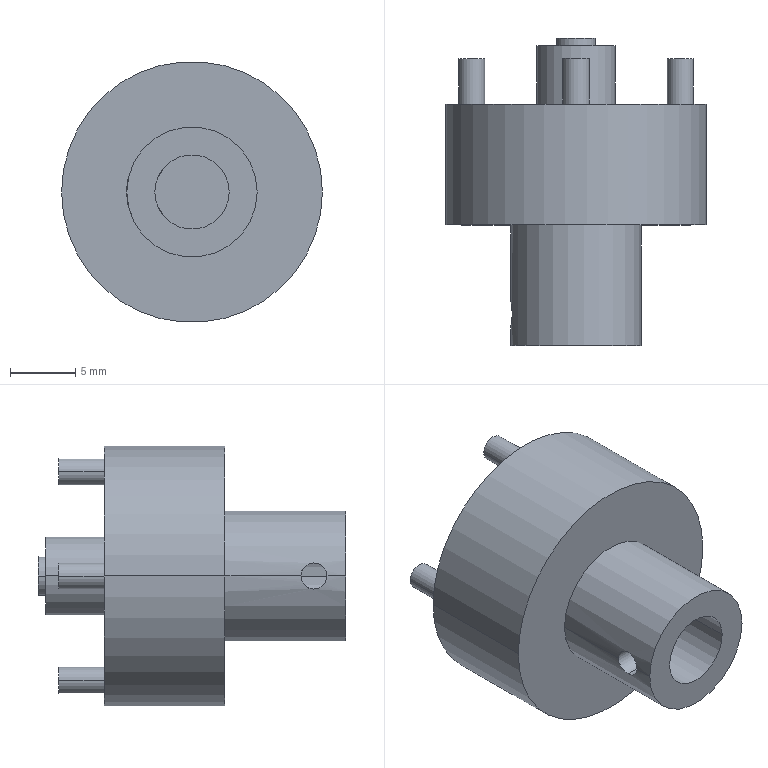Part | SolidWorks | features BaseBody 1 | 1 solid | 30 faces | box 20 x 23.55 x 20 mm | volume 3677 mm3 | cylinder 20 | plane 10 | commonest cylinder face diameters 2 x10 3 x2 5.7 x2 6 x2 10 x2 20 x2
STEP:
#1=CARTESIAN_POINT('',(7.,12.825,0.));
#2=VERTEX_POINT('',#1);
#3=CARTESIAN_POINT('',(9.,12.825,0.));
#4=VERTEX_POINT('',#3);
#5=CARTESIAN_POINT('',(8.,12.825,0.));
#6=DIRECTION('',(0.,1.,0.));
#7=DIRECTION('',(-1.,0.,0.));
#8=AXIS2_PLACEMENT_3D('',#5,#6,#7);
#9=CIRCLE('',#8,1.);
#10=EDGE_CURVE('',#2,#4,#9,.T.);
#11=ORIENTED_EDGE('',*,*,#10,.F.);
#12=CARTESIAN_POINT('',(7.,9.325,0.));
#13=VERTEX_POINT('',#12);
#14=CARTESIAN_POINT('',(7.,12.825,0.));
#15=DIRECTION('',(0.,-1.,0.));
#16=VECTOR('',#15,1000.);
#17=LINE('',#14,#16);
#18=EDGE_CURVE('',#2,#13,#17,.T.);
#19=ORIENTED_EDGE('',*,*,#18,.T.);
#20=CARTESIAN_POINT('',(9.,9.325,0.));
#21=VERTEX_POINT('',#20);
#22=CARTESIAN_POINT('',(8.,9.325,0.));
#23=DIRECTION('',(0.,1.,0.));
#24=DIRECTION('',(-1.,0.,0.));
#25=AXIS2_PLACEMENT_3D('',#22,#23,#24);
#26=CIRCLE('',#25,1.);
#27=EDGE_CURVE('',#13,#21,#26,.T.);
#28=ORIENTED_EDGE('',*,*,#27,.T.);
#29=CARTESIAN_POINT('',(9.,12.825,0.));
#30=DIRECTION('',(0.,-1.,0.));
#31=VECTOR('',#30,1000.);
#32=LINE('',#29,#31);
#33=EDGE_CURVE('',#4,#21,#32,.T.);
#34=ORIENTED_EDGE('',*,*,#33,.F.);
#35=EDGE_LOOP('',(#11,#19,#28,#34));
#36=FACE_OUTER_BOUND('',#35,.T.);
#37=CARTESIAN_POINT('',(8.,12.825,0.));
#38=DIRECTION('',(0.,-1.,0.));
#39=DIRECTION('',(1.,0.,0.));
#40=AXIS2_PLACEMENT_3D('',#37,#38,#39);
#41=CYLINDRICAL_SURFACE('',#40,1.);
#42=ADVANCED_FACE('',(#36),#41,.T.);
#43=CARTESIAN_POINT('',(-1.,12.825,-8.));
#44=VERTEX_POINT('',#43);
#45=CARTESIAN_POINT('',(1.,12.825,-8.));
#46=VERTEX_POINT('',#45);
#47=CARTESIAN_POINT('',(0.,12.825,-8.));
#48=DIRECTION('',(0.,1.,0.));
#49=DIRECTION('',(-1.,0.,0.));
#50=AXIS2_PLACEMENT_3D('',#47,#48,#49);
#51=CIRCLE('',#50,1.);
#52=EDGE_CURVE('',#44,#46,#51,.T.);
#53=ORIENTED_EDGE('',*,*,#52,.F.);
#54=CARTESIAN_POINT('',(-1.,9.325,-8.));
#55=VERTEX_POINT('',#54);
#56=CARTESIAN_POINT('',(-1.,12.825,-8.));
#57=DIRECTION('',(0.,-1.,0.));
#58=VECTOR('',#57,1000.);
#59=LINE('',#56,#58);
#60=EDGE_CURVE('',#44,#55,#59,.T.);
#61=ORIENTED_EDGE('',*,*,#60,.T.);
#62=CARTESIAN_POINT('',(1.,9.325,-8.));
#63=VERTEX_POINT('',#62);
#64=CARTESIAN_POINT('',(0.,9.325,-8.));
#65=DIRECTION('',(0.,1.,0.));
#66=DIRECTION('',(-1.,0.,0.));
#67=AXIS2_PLACEMENT_3D('',#64,#65,#66);
#68=CIRCLE('',#67,1.);
#69=EDGE_CURVE('',#55,#63,#68,.T.);
#70=ORIENTED_EDGE('',*,*,#69,.T.);
#71=CARTESIAN_POINT('',(1.,12.825,-8.));
#72=DIRECTION('',(0.,-1.,0.));
#73=VECTOR('',#72,1000.);
#74=LINE('',#71,#73);
#75=EDGE_CURVE('',#46,#63,#74,.T.);
#76=ORIENTED_EDGE('',*,*,#75,.F.);
#77=EDGE_LOOP('',(#53,#61,#70,#76));
#78=FACE_OUTER_BOUND('',#77,.T.);
#79=CARTESIAN_POINT('',(0.,12.825,-8.));
#80=DIRECTION('',(0.,-1.,0.));
#81=DIRECTION('',(1.,0.,0.));
#82=AXIS2_PLACEMENT_3D('',#79,#80,#81);
#83=CYLINDRICAL_SURFACE('',#82,1.);
#84=ADVANCED_FACE('',(#78),#83,.T.);
#85=CARTESIAN_POINT('',(-9.,12.825,0.));
#86=VERTEX_POINT('',#85);
#87=CARTESIAN_POINT('',(-7.,12.825,0.));
#88=VERTEX_POINT('',#87);
#89=CARTESIAN_POINT('',(-8.,12.825,0.));
#90=DIRECTION('',(0.,1.,0.));
#91=DIRECTION('',(-1.,0.,0.));
#92=AXIS2_PLACEMENT_3D('',#89,#90,#91);
#93=CIRCLE('',#92,1.);
#94=EDGE_CURVE('',#86,#88,#93,.T.);
#95=ORIENTED_EDGE('',*,*,#94,.F.);
#96=CARTESIAN_POINT('',(-9.,9.325,0.));
#97=VERTEX_POINT('',#96);
#98=CARTESIAN_POINT('',(-9.,12.825,0.));
#99=DIRECTION('',(0.,-1.,0.));
#100=VECTOR('',#99,1000.);
#101=LINE('',#98,#100);
#102=EDGE_CURVE('',#86,#97,#101,.T.);
#103=ORIENTED_EDGE('',*,*,#102,.T.);
#104=CARTESIAN_POINT('',(-7.,9.325,0.));
#105=VERTEX_POINT('',#104);
#106=CARTESIAN_POINT('',(-8.,9.325,0.));
#107=DIRECTION('',(0.,1.,0.));
#108=DIRECTION('',(-1.,0.,0.));
#109=AXIS2_PLACEMENT_3D('',#106,#107,#108);
#110=CIRCLE('',#109,1.);
#111=EDGE_CURVE('',#97,#105,#110,.T.);
#112=ORIENTED_EDGE('',*,*,#111,.T.);
#113=CARTESIAN_POINT('',(-7.,12.825,0.));
#114=DIRECTION('',(0.,-1.,0.));
#115=VECTOR('',#114,1000.);
#116=LINE('',#113,#115);
#117=EDGE_CURVE('',#88,#105,#116,.T.);
#118=ORIENTED_EDGE('',*,*,#117,.F.);
#119=EDGE_LOOP('',(#95,#103,#112,#118));
#120=FACE_OUTER_BOUND('',#119,.T.);
#121=CARTESIAN_POINT('',(-8.,12.825,0.));
#122=DIRECTION('',(0.,-1.,0.));
#123=DIRECTION('',(1.,0.,0.));
#124=AXIS2_PLACEMENT_3D('',#121,#122,#123);
#125=CYLINDRICAL_SURFACE('',#124,1.);
#126=ADVANCED_FACE('',(#120),#125,.T.);
#127=CARTESIAN_POINT('',(-1.,12.825,8.));
#128=VERTEX_POINT('',#127);
#129=CARTESIAN_POINT('',(1.,12.825,8.));
#130=VERTEX_POINT('',#129);
#131=CARTESIAN_POINT('',(0.,12.825,8.));
#132=DIRECTION('',(0.,1.,0.));
#133=DIRECTION('',(-1.,0.,0.));
#134=AXIS2_PLACEMENT_3D('',#131,#132,#133);
#135=CIRCLE('',#134,1.);
#136=EDGE_CURVE('',#128,#130,#135,.T.);
#137=ORIENTED_EDGE('',*,*,#136,.F.);
#138=CARTESIAN_POINT('',(-1.,9.325,8.));
#139=VERTEX_POINT('',#138);
#140=CARTESIAN_POINT('',(-1.,12.825,8.));
#141=DIRECTION('',(0.,-1.,0.));
#142=VECTOR('',#141,1000.);
#143=LINE('',#140,#142);
#144=EDGE_CURVE('',#128,#139,#143,.T.);
#145=ORIENTED_EDGE('',*,*,#144,.T.);
#146=CARTESIAN_POINT('',(1.,9.325,8.));
#147=VERTEX_POINT('',#146);
#148=CARTESIAN_POINT('',(0.,9.325,8.));
#149=DIRECTION('',(0.,1.,0.));
#150=DIRECTION('',(-1.,0.,0.));
#151=AXIS2_PLACEMENT_3D('',#148,#149,#150);
#152=CIRCLE('',#151,1.);
#153=EDGE_CURVE('',#139,#147,#152,.T.);
#154=ORIENTED_EDGE('',*,*,#153,.T.);
#155=CARTESIAN_POINT('',(1.,12.825,8.));
#156=DIRECTION('',(0.,-1.,0.));
#157=VECTOR('',#156,1000.);
#158=LINE('',#155,#157);
#159=EDGE_CURVE('',#130,#147,#158,.T.);
#160=ORIENTED_EDGE('',*,*,#159,.F.);
#161=EDGE_LOOP('',(#137,#145,#154,#160));
#162=FACE_OUTER_BOUND('',#161,.T.);
#163=CARTESIAN_POINT('',(0.,12.825,8.));
#164=DIRECTION('',(0.,-1.,0.));
#165=DIRECTION('',(1.,0.,0.));
#166=AXIS2_PLACEMENT_3D('',#163,#164,#165);
#167=CYLINDRICAL_SURFACE('',#166,1.);
#168=ADVANCED_FACE('',(#162),#167,.T.);
#169=CARTESIAN_POINT('',(-5.,-7.75,0.));
#170=VERTEX_POINT('',#169);
#171=CARTESIAN_POINT('',(-4.899,-6.75,1.));
#172=VERTEX_POINT('',#171);
#173=CARTESIAN_POINT('',(-5.,-7.75,0.));
#174=CARTESIAN_POINT('',(-5.,-7.75,0.1308));
#175=CARTESIAN_POINT('',(-4.995,-7.724,0.262));
#176=CARTESIAN_POINT('',(-4.976,-7.623,0.5045));
#177=CARTESIAN_POINT('',(-4.963,-7.55,0.6144));
#178=CARTESIAN_POINT('',(-4.936,-7.364,0.8002));
#179=CARTESIAN_POINT('',(-4.923,-7.254,0.8737));
#180=CARTESIAN_POINT('',(-4.905,-7.012,0.9739));
#181=CARTESIAN_POINT('',(-4.899,-6.881,1.));
#182=CARTESIAN_POINT('',(-4.899,-6.75,1.));
#183=B_SPLINE_CURVE_WITH_KNOTS('',3,(#173,#174,#175,#176,#177,#178,#179,#180,#181,#182),.UNSPECIFIED.,.F.,.F.,(4,2,2,2,4),(0.001568,0.001959,0.002351,0.002743,0.003134),.UNSPECIFIED.);
#184=EDGE_CURVE('',#170,#172,#183,.T.);
#185=ORIENTED_EDGE('',*,*,#184,.T.);
#186=CARTESIAN_POINT('',(-2.669,-6.75,1.));
#187=VERTEX_POINT('',#186);
#188=CARTESIAN_POINT('',(-11.,-6.75,1.));
#189=DIRECTION('',(1.,0.,0.));
#190=VECTOR('',#189,1000.);
#191=LINE('',#188,#190);
#192=EDGE_CURVE('',#172,#187,#191,.T.);
#193=ORIENTED_EDGE('',*,*,#192,.T.);
#194=CARTESIAN_POINT('',(-2.85,-7.75,0.));
#195=VERTEX_POINT('',#194);
#196=CARTESIAN_POINT('',(-2.669,-6.75,1.));
#197=CARTESIAN_POINT('',(-2.669,-6.881,1.));
#198=CARTESIAN_POINT('',(-2.679,-7.014,0.9734));
#199=CARTESIAN_POINT('',(-2.714,-7.255,0.873));
#200=CARTESIAN_POINT('',(-2.737,-7.365,0.7995));
#201=CARTESIAN_POINT('',(-2.785,-7.549,0.6148));
#202=CARTESIAN_POINT('',(-2.807,-7.623,0.5057));
#203=CARTESIAN_POINT('',(-2.84,-7.724,0.263));
#204=CARTESIAN_POINT('',(-2.85,-7.75,0.1318));
#205=CARTESIAN_POINT('',(-2.85,-7.75,0.));
#206=B_SPLINE_CURVE_WITH_KNOTS('',3,(#196,#197,#198,#199,#200,#201,#202,#203,#204,#205),.UNSPECIFIED.,.F.,.F.,(4,2,2,2,4),(0.003152,0.003545,0.003939,0.004333,0.004727),.UNSPECIFIED.);
#207=EDGE_CURVE('',#187,#195,#206,.T.);
#208=ORIENTED_EDGE('',*,*,#207,.T.);
#209=CARTESIAN_POINT('',(-2.669,-6.75,-1.));
#210=VERTEX_POINT('',#209);
#211=CARTESIAN_POINT('',(-2.85,-7.75,0.));
#212=CARTESIAN_POINT('',(-2.85,-7.75,-0.1318));
#213=CARTESIAN_POINT('',(-2.84,-7.723,-0.2641));
#214=CARTESIAN_POINT('',(-2.808,-7.623,-0.505));
#215=CARTESIAN_POINT('',(-2.784,-7.549,-0.6156));
#216=CARTESIAN_POINT('',(-2.737,-7.365,-0.7989));
#217=CARTESIAN_POINT('',(-2.714,-7.256,-0.8727));
#218=CARTESIAN_POINT('',(-2.679,-7.013,-0.9735));
#219=CARTESIAN_POINT('',(-2.669,-6.883,-1.));
#220=CARTESIAN_POINT('',(-2.669,-6.75,-1.));
#221=B_SPLINE_CURVE_WITH_KNOTS('',3,(#211,#212,#213,#214,#215,#216,#217,#218,#219,#220),.UNSPECIFIED.,.F.,.F.,(4,2,2,2,4),(0.004727,0.005121,0.005515,0.005909,0.006303),.UNSPECIFIED.);
#222=EDGE_CURVE('',#195,#210,#221,.T.);
#223=ORIENTED_EDGE('',*,*,#222,.T.);
#224=CARTESIAN_POINT('',(-4.899,-6.75,-1.));
#225=VERTEX_POINT('',#224);
#226=CARTESIAN_POINT('',(-11.,-6.75,-1.));
#227=DIRECTION('',(1.,0.,0.));
#228=VECTOR('',#227,1000.);
#229=LINE('',#226,#228);
#230=EDGE_CURVE('',#225,#210,#229,.T.);
#231=ORIENTED_EDGE('',*,*,#230,.F.);
#232=CARTESIAN_POINT('',(-4.899,-6.75,-1.));
#233=CARTESIAN_POINT('',(-4.899,-6.883,-1.));
#234=CARTESIAN_POINT('',(-4.905,-7.013,-0.9738));
#235=CARTESIAN_POINT('',(-4.923,-7.255,-0.8732));
#236=CARTESIAN_POINT('',(-4.937,-7.365,-0.7989));
#237=CARTESIAN_POINT('',(-4.963,-7.549,-0.6148));
#238=CARTESIAN_POINT('',(-4.976,-7.624,-0.5034));
#239=CARTESIAN_POINT('',(-4.995,-7.724,-0.2627));
#240=CARTESIAN_POINT('',(-5.,-7.75,-0.1309));
#241=CARTESIAN_POINT('',(-5.,-7.75,0.));
#242=B_SPLINE_CURVE_WITH_KNOTS('',3,(#232,#233,#234,#235,#236,#237,#238,#239,#240,#241),.UNSPECIFIED.,.F.,.F.,(4,2,2,2,4),(0.,0.0003919,0.0007838,0.001176,0.001568),.UNSPECIFIED.);
#243=EDGE_CURVE('',#225,#170,#242,.T.);
#244=ORIENTED_EDGE('',*,*,#243,.T.);
#245=EDGE_LOOP('',(#185,#193,#208,#223,#231,#244));
#246=FACE_OUTER_BOUND('',#245,.T.);
#247=CARTESIAN_POINT('',(-11.,-6.75,0.));
#248=DIRECTION('',(1.,0.,0.));
#249=DIRECTION('',(0.,0.,-1.));
#250=AXIS2_PLACEMENT_3D('',#247,#248,#249);
#251=CYLINDRICAL_SURFACE('',#250,1.);
#252=ADVANCED_FACE('',(#246),#251,.F.);
#253=CARTESIAN_POINT('',(-2.85,-4.325,0.));
#254=VERTEX_POINT('',#253);
#255=CARTESIAN_POINT('',(2.85,-4.325,0.));
#256=VERTEX_POINT('',#255);
#257=CARTESIAN_POINT('',(0.,-4.325,0.));
#258=DIRECTION('',(0.,-1.,0.));
#259=DIRECTION('',(1.,0.,0.));
#260=AXIS2_PLACEMENT_3D('',#257,#258,#259);
#261=CIRCLE('',#260,2.85);
#262=EDGE_CURVE('',#254,#256,#261,.T.);
#263=ORIENTED_EDGE('',*,*,#262,.F.);
#264=CARTESIAN_POINT('',(-2.85,-5.75,0.));
#265=VERTEX_POINT('',#264);
#266=CARTESIAN_POINT('',(-2.85,-4.325,0.));
#267=DIRECTION('',(0.,-1.,0.));
#268=VECTOR('',#267,1000.);
#269=LINE('',#266,#268);
#270=EDGE_CURVE('',#254,#265,#269,.T.);
#271=ORIENTED_EDGE('',*,*,#270,.T.);
#272=CARTESIAN_POINT('',(-2.669,-6.75,-1.));
#273=CARTESIAN_POINT('',(-2.669,-6.617,-1.));
#274=CARTESIAN_POINT('',(-2.679,-6.486,-0.9734));
#275=CARTESIAN_POINT('',(-2.714,-6.244,-0.8726));
#276=CARTESIAN_POINT('',(-2.738,-6.134,-0.7984));
#277=CARTESIAN_POINT('',(-2.784,-5.951,-0.6153));
#278=CARTESIAN_POINT('',(-2.808,-5.877,-0.5046));
#279=CARTESIAN_POINT('',(-2.84,-5.777,-0.2641));
#280=CARTESIAN_POINT('',(-2.85,-5.75,-0.1317));
#281=CARTESIAN_POINT('',(-2.85,-5.75,0.));
#282=B_SPLINE_CURVE_WITH_KNOTS('',3,(#272,#273,#274,#275,#276,#277,#278,#279,#280,#281),.UNSPECIFIED.,.F.,.F.,(4,2,2,2,4),(0.,0.0003941,0.0007881,0.001182,0.001576),.UNSPECIFIED.);
#283=EDGE_CURVE('',#210,#265,#282,.T.);
#284=ORIENTED_EDGE('',*,*,#283,.F.);
#285=ORIENTED_EDGE('',*,*,#222,.F.);
#286=CARTESIAN_POINT('',(-2.85,-9.175,0.));
#287=VERTEX_POINT('',#286);
#288=CARTESIAN_POINT('',(-2.85,-4.325,0.));
#289=DIRECTION('',(0.,-1.,0.));
#290=VECTOR('',#289,1000.);
#291=LINE('',#288,#290);
#292=EDGE_CURVE('',#195,#287,#291,.T.);
#293=ORIENTED_EDGE('',*,*,#292,.T.);
#294=CARTESIAN_POINT('',(2.85,-9.175,0.));
#295=VERTEX_POINT('',#294);
#296=CARTESIAN_POINT('',(0.,-9.175,0.));
#297=DIRECTION('',(0.,-1.,0.));
#298=DIRECTION('',(1.,0.,0.));
#299=AXIS2_PLACEMENT_3D('',#296,#297,#298);
#300=CIRCLE('',#299,2.85);
#301=EDGE_CURVE('',#287,#295,#300,.T.);
#302=ORIENTED_EDGE('',*,*,#301,.T.);
#303=CARTESIAN_POINT('',(2.85,-4.325,0.));
#304=DIRECTION('',(0.,-1.,0.));
#305=VECTOR('',#304,1000.);
#306=LINE('',#303,#305);
#307=EDGE_CURVE('',#256,#295,#306,.T.);
#308=ORIENTED_EDGE('',*,*,#307,.F.);
#309=EDGE_LOOP('',(#263,#271,#284,#285,#293,#302,#308));
#310=FACE_OUTER_BOUND('',#309,.T.);
#311=CARTESIAN_POINT('',(0.,-4.325,0.));
#312=DIRECTION('',(0.,-1.,0.));
#313=DIRECTION('',(1.,0.,0.));
#314=AXIS2_PLACEMENT_3D('',#311,#312,#313);
#315=CYLINDRICAL_SURFACE('',#314,2.85);
#316=ADVANCED_FACE('',(#310),#315,.F.);
#317=CARTESIAN_POINT('',(5.,0.075,0.));
#318=VERTEX_POINT('',#317);
#319=CARTESIAN_POINT('',(-5.,0.075,0.));
#320=VERTEX_POINT('',#319);
#321=CARTESIAN_POINT('',(0.,0.075,0.));
#322=DIRECTION('',(0.,-1.,0.));
#323=DIRECTION('',(1.,0.,0.));
#324=AXIS2_PLACEMENT_3D('',#321,#322,#323);
#325=CIRCLE('',#324,5.);
#326=EDGE_CURVE('',#318,#320,#325,.T.);
#327=ORIENTED_EDGE('',*,*,#326,.T.);
#328=CARTESIAN_POINT('',(-5.,-5.75,0.));
#329=VERTEX_POINT('',#328);
#330=CARTESIAN_POINT('',(-5.,-4.325,0.));
#331=DIRECTION('',(0.,-1.,0.));
#332=VECTOR('',#331,1000.);
#333=LINE('',#330,#332);
#334=EDGE_CURVE('',#320,#329,#333,.T.);
#335=ORIENTED_EDGE('',*,*,#334,.T.);
#336=CARTESIAN_POINT('',(-4.899,-6.75,1.));
#337=CARTESIAN_POINT('',(-4.899,-6.619,1.));
#338=CARTESIAN_POINT('',(-4.905,-6.487,0.9737));
#339=CARTESIAN_POINT('',(-4.923,-6.247,0.8738));
#340=CARTESIAN_POINT('',(-4.937,-6.135,0.7995));
#341=CARTESIAN_POINT('',(-4.963,-5.951,0.6152));
#342=CARTESIAN_POINT('',(-4.976,-5.877,0.505));
#343=CARTESIAN_POINT('',(-4.995,-5.776,0.2622));
#344=CARTESIAN_POINT('',(-5.,-5.75,0.1321));
#345=CARTESIAN_POINT('',(-5.,-5.75,0.));
#346=B_SPLINE_CURVE_WITH_KNOTS('',3,(#336,#337,#338,#339,#340,#341,#342,#343,#344,#345),.UNSPECIFIED.,.F.,.F.,(4,2,2,2,4),(0.003134,0.003526,0.003918,0.00431,0.004702),.UNSPECIFIED.);
#347=EDGE_CURVE('',#172,#329,#346,.T.);
#348=ORIENTED_EDGE('',*,*,#347,.F.);
#349=ORIENTED_EDGE('',*,*,#184,.F.);
#350=CARTESIAN_POINT('',(-5.,-9.175,0.));
#351=VERTEX_POINT('',#350);
#352=CARTESIAN_POINT('',(-5.,-4.325,0.));
#353=DIRECTION('',(0.,-1.,0.));
#354=VECTOR('',#353,1000.);
#355=LINE('',#352,#354);
#356=EDGE_CURVE('',#170,#351,#355,.T.);
#357=ORIENTED_EDGE('',*,*,#356,.T.);
#358=CARTESIAN_POINT('',(5.,-9.175,0.));
#359=VERTEX_POINT('',#358);
#360=CARTESIAN_POINT('',(0.,-9.175,0.));
#361=DIRECTION('',(0.,-1.,0.));
#362=DIRECTION('',(1.,0.,0.));
#363=AXIS2_PLACEMENT_3D('',#360,#361,#362);
#364=CIRCLE('',#363,5.);
#365=EDGE_CURVE('',#359,#351,#364,.T.);
#366=ORIENTED_EDGE('',*,*,#365,.F.);
#367=CARTESIAN_POINT('',(5.,-4.325,0.));
#368=DIRECTION('',(0.,-1.,0.));
#369=VECTOR('',#368,1000.);
#370=LINE('',#367,#369);
#371=EDGE_CURVE('',#318,#359,#370,.T.);
#372=ORIENTED_EDGE('',*,*,#371,.F.);
#373=EDGE_LOOP('',(#327,#335,#348,#349,#357,#366,#372));
#374=FACE_OUTER_BOUND('',#373,.T.);
#375=CARTESIAN_POINT('',(0.,-4.325,0.));
#376=DIRECTION('',(0.,-1.,0.));
#377=DIRECTION('',(1.,0.,0.));
#378=AXIS2_PLACEMENT_3D('',#375,#376,#377);
#379=CYLINDRICAL_SURFACE('',#378,5.);
#380=ADVANCED_FACE('',(#374),#379,.T.);
#381=CARTESIAN_POINT('',(10.,9.325,0.));
#382=VERTEX_POINT('',#381);
#383=CARTESIAN_POINT('',(-10.,9.325,0.));
#384=VERTEX_POINT('',#383);
#385=CARTESIAN_POINT('',(0.,9.325,0.));
#386=DIRECTION('',(0.,-1.,0.));
#387=DIRECTION('',(1.,0.,0.));
#388=AXIS2_PLACEMENT_3D('',#385,#386,#387);
#389=CIRCLE('',#388,10.);
#390=EDGE_CURVE('',#382,#384,#389,.T.);
#391=ORIENTED_EDGE('',*,*,#390,.T.);
#392=CARTESIAN_POINT('',(-10.,0.075,0.));
#393=VERTEX_POINT('',#392);
#394=CARTESIAN_POINT('',(-10.,-4.325,0.));
#395=DIRECTION('',(0.,-1.,0.));
#396=VECTOR('',#395,1000.);
#397=LINE('',#394,#396);
#398=EDGE_CURVE('',#384,#393,#397,.T.);
#399=ORIENTED_EDGE('',*,*,#398,.T.);
#400=CARTESIAN_POINT('',(10.,0.075,0.));
#401=VERTEX_POINT('',#400);
#402=CARTESIAN_POINT('',(0.,0.075,0.));
#403=DIRECTION('',(0.,-1.,0.));
#404=DIRECTION('',(1.,0.,0.));
#405=AXIS2_PLACEMENT_3D('',#402,#403,#404);
#406=CIRCLE('',#405,10.);
#407=EDGE_CURVE('',#401,#393,#406,.T.);
#408=ORIENTED_EDGE('',*,*,#407,.F.);
#409=CARTESIAN_POINT('',(10.,-4.325,0.));
#410=DIRECTION('',(0.,-1.,0.));
#411=VECTOR('',#410,1000.);
#412=LINE('',#409,#411);
#413=EDGE_CURVE('',#382,#401,#412,.T.);
#414=ORIENTED_EDGE('',*,*,#413,.F.);
#415=EDGE_LOOP('',(#391,#399,#408,#414));
#416=FACE_OUTER_BOUND('',#415,.T.);
#417=CARTESIAN_POINT('',(0.,-4.325,0.));
#418=DIRECTION('',(0.,-1.,0.));
#419=DIRECTION('',(1.,0.,0.));
#420=AXIS2_PLACEMENT_3D('',#417,#418,#419);
#421=CYLINDRICAL_SURFACE('',#420,10.);
#422=ADVANCED_FACE('',(#416),#421,.T.);
#423=CARTESIAN_POINT('',(3.,13.825,0.));
#424=VERTEX_POINT('',#423);
#425=CARTESIAN_POINT('',(-3.,13.825,0.));
#426=VERTEX_POINT('',#425);
#427=CARTESIAN_POINT('',(0.,13.825,0.));
#428=DIRECTION('',(0.,-1.,0.));
#429=DIRECTION('',(1.,0.,0.));
#430=AXIS2_PLACEMENT_3D('',#427,#428,#429);
#431=CIRCLE('',#430,3.);
#432=EDGE_CURVE('',#424,#426,#431,.T.);
#433=ORIENTED_EDGE('',*,*,#432,.T.);
#434=CARTESIAN_POINT('',(-3.,9.325,0.));
#435=VERTEX_POINT('',#434);
#436=CARTESIAN_POINT('',(-3.,-4.325,0.));
#437=DIRECTION('',(0.,-1.,0.));
#438=VECTOR('',#437,1000.);
#439=LINE('',#436,#438);
#440=EDGE_CURVE('',#426,#435,#439,.T.);
#441=ORIENTED_EDGE('',*,*,#440,.T.);
#442=CARTESIAN_POINT('',(3.,9.325,0.));
#443=VERTEX_POINT('',#442);
#444=CARTESIAN_POINT('',(0.,9.325,0.));
#445=DIRECTION('',(0.,-1.,0.));
#446=DIRECTION('',(1.,0.,0.));
#447=AXIS2_PLACEMENT_3D('',#444,#445,#446);
#448=CIRCLE('',#447,3.);
#449=EDGE_CURVE('',#443,#435,#448,.T.);
#450=ORIENTED_EDGE('',*,*,#449,.F.);
#451=CARTESIAN_POINT('',(3.,-4.325,0.));
#452=DIRECTION('',(0.,-1.,0.));
#453=VECTOR('',#452,1000.);
#454=LINE('',#451,#453);
#455=EDGE_CURVE('',#424,#443,#454,.T.);
#456=ORIENTED_EDGE('',*,*,#455,.F.);
#457=EDGE_LOOP('',(#433,#441,#450,#456));
#458=FACE_OUTER_BOUND('',#457,.T.);
#459=CARTESIAN_POINT('',(0.,-4.325,0.));
#460=DIRECTION('',(0.,-1.,0.));
#461=DIRECTION('',(1.,0.,0.));
#462=AXIS2_PLACEMENT_3D('',#459,#460,#461);
#463=CYLINDRICAL_SURFACE('',#462,3.);
#464=ADVANCED_FACE('',(#458),#463,.T.);
#465=CARTESIAN_POINT('',(1.5,14.375,0.));
#466=VERTEX_POINT('',#465);
#467=CARTESIAN_POINT('',(-1.5,14.375,0.));
#468=VERTEX_POINT('',#467);
#469=CARTESIAN_POINT('',(0.,14.375,0.));
#470=DIRECTION('',(0.,-1.,0.));
#471=DIRECTION('',(1.,0.,0.));
#472=AXIS2_PLACEMENT_3D('',#469,#470,#471);
#473=CIRCLE('',#472,1.5);
#474=EDGE_CURVE('',#466,#468,#473,.T.);
#475=ORIENTED_EDGE('',*,*,#474,.T.);
#476=CARTESIAN_POINT('',(-1.5,13.825,0.));
#477=VERTEX_POINT('',#476);
#478=CARTESIAN_POINT('',(-1.5,-4.325,0.));
#479=DIRECTION('',(0.,-1.,0.));
#480=VECTOR('',#479,1000.);
#481=LINE('',#478,#480);
#482=EDGE_CURVE('',#468,#477,#481,.T.);
#483=ORIENTED_EDGE('',*,*,#482,.T.);
#484=CARTESIAN_POINT('',(1.5,13.825,0.));
#485=VERTEX_POINT('',#484);
#486=CARTESIAN_POINT('',(0.,13.825,0.));
#487=DIRECTION('',(0.,-1.,0.));
#488=DIRECTION('',(1.,0.,0.));
#489=AXIS2_PLACEMENT_3D('',#486,#487,#488);
#490=CIRCLE('',#489,1.5);
#491=EDGE_CURVE('',#485,#477,#490,.T.);
#492=ORIENTED_EDGE('',*,*,#491,.F.);
#493=CARTESIAN_POINT('',(1.5,-4.325,0.));
#494=DIRECTION('',(0.,-1.,0.));
#495=VECTOR('',#494,1000.);
#496=LINE('',#493,#495);
#497=EDGE_CURVE('',#466,#485,#496,.T.);
#498=ORIENTED_EDGE('',*,*,#497,.F.);
#499=EDGE_LOOP('',(#475,#483,#492,#498));
#500=FACE_OUTER_BOUND('',#499,.T.);
#501=CARTESIAN_POINT('',(0.,-4.325,0.));
#502=DIRECTION('',(0.,-1.,0.));
#503=DIRECTION('',(1.,0.,0.));
#504=AXIS2_PLACEMENT_3D('',#501,#502,#503);
#505=CYLINDRICAL_SURFACE('',#504,1.5);
#506=ADVANCED_FACE('',(#500),#505,.T.);
#507=ORIENTED_EDGE('',*,*,#474,.F.);
#508=CARTESIAN_POINT('',(0.,14.375,0.));
#509=DIRECTION('',(0.,-1.,0.));
#510=DIRECTION('',(1.,0.,0.));
#511=AXIS2_PLACEMENT_3D('',#508,#509,#510);
#512=CIRCLE('',#511,1.5);
#513=EDGE_CURVE('',#468,#466,#512,.T.);
#514=ORIENTED_EDGE('',*,*,#513,.F.);
#515=EDGE_LOOP('',(#507,#514));
#516=FACE_OUTER_BOUND('',#515,.T.);
#517=CARTESIAN_POINT('',(0.,14.375,0.));
#518=DIRECTION('',(0.,1.,0.));
#519=DIRECTION('',(-1.,0.,0.));
#520=AXIS2_PLACEMENT_3D('',#517,#518,#519);
#521=PLANE('',#520);
#522=ADVANCED_FACE('',(#516),#521,.T.);
#523=ORIENTED_EDGE('',*,*,#482,.F.);
#524=ORIENTED_EDGE('',*,*,#513,.T.);
#525=ORIENTED_EDGE('',*,*,#497,.T.);
#526=CARTESIAN_POINT('',(0.,13.825,0.));
#527=DIRECTION('',(0.,-1.,0.));
#528=DIRECTION('',(1.,0.,0.));
#529=AXIS2_PLACEMENT_3D('',#526,#527,#528);
#530=CIRCLE('',#529,1.5);
#531=EDGE_CURVE('',#477,#485,#530,.T.);
#532=ORIENTED_EDGE('',*,*,#531,.F.);
#533=EDGE_LOOP('',(#523,#524,#525,#532));
#534=FACE_OUTER_BOUND('',#533,.T.);
#535=CARTESIAN_POINT('',(0.,-4.325,0.));
#536=DIRECTION('',(0.,-1.,0.));
#537=DIRECTION('',(1.,0.,0.));
#538=AXIS2_PLACEMENT_3D('',#535,#536,#537);
#539=CYLINDRICAL_SURFACE('',#538,1.5);
#540=ADVANCED_FACE('',(#534),#539,.T.);
#541=ORIENTED_EDGE('',*,*,#491,.T.);
#542=ORIENTED_EDGE('',*,*,#531,.T.);
#543=EDGE_LOOP('',(#541,#542));
#544=FACE_BOUND('',#543,.T.);
#545=ORIENTED_EDGE('',*,*,#432,.F.);
#546=CARTESIAN_POINT('',(0.,13.825,0.));
#547=DIRECTION('',(0.,-1.,0.));
#548=DIRECTION('',(1.,0.,0.));
#549=AXIS2_PLACEMENT_3D('',#546,#547,#548);
#550=CIRCLE('',#549,3.);
#551=EDGE_CURVE('',#426,#424,#550,.T.);
#552=ORIENTED_EDGE('',*,*,#551,.F.);
#553=EDGE_LOOP('',(#545,#552));
#554=FACE_OUTER_BOUND('',#553,.T.);
#555=CARTESIAN_POINT('',(1.5,13.825,0.));
#556=DIRECTION('',(0.,1.,0.));
#557=DIRECTION('',(-1.,0.,0.));
#558=AXIS2_PLACEMENT_3D('',#555,#556,#557);
#559=PLANE('',#558);
#560=ADVANCED_FACE('',(#544,#554),#559,.T.);
#561=ORIENTED_EDGE('',*,*,#440,.F.);
#562=ORIENTED_EDGE('',*,*,#551,.T.);
#563=ORIENTED_EDGE('',*,*,#455,.T.);
#564=CARTESIAN_POINT('',(0.,9.325,0.));
#565=DIRECTION('',(0.,-1.,0.));
#566=DIRECTION('',(1.,0.,0.));
#567=AXIS2_PLACEMENT_3D('',#564,#565,#566);
#568=CIRCLE('',#567,3.);
#569=EDGE_CURVE('',#435,#443,#568,.T.);
#570=ORIENTED_EDGE('',*,*,#569,.F.);
#571=EDGE_LOOP('',(#561,#562,#563,#570));
#572=FACE_OUTER_BOUND('',#571,.T.);
#573=CARTESIAN_POINT('',(0.,-4.325,0.));
#574=DIRECTION('',(0.,-1.,0.));
#575=DIRECTION('',(1.,0.,0.));
#576=AXIS2_PLACEMENT_3D('',#573,#574,#575);
#577=CYLINDRICAL_SURFACE('',#576,3.);
#578=ADVANCED_FACE('',(#572),#577,.T.);
#579=CARTESIAN_POINT('',(8.,9.325,0.));
#580=DIRECTION('',(0.,1.,0.));
#581=DIRECTION('',(-1.,0.,0.));
#582=AXIS2_PLACEMENT_3D('',#579,#580,#581);
#583=CIRCLE('',#582,1.);
#584=EDGE_CURVE('',#21,#13,#583,.T.);
#585=ORIENTED_EDGE('',*,*,#584,.F.);
#586=ORIENTED_EDGE('',*,*,#27,.F.);
#587=EDGE_LOOP('',(#585,#586));
#588=FACE_BOUND('',#587,.T.);
#589=CARTESIAN_POINT('',(0.,9.325,-8.));
#590=DIRECTION('',(0.,1.,0.));
#591=DIRECTION('',(-1.,0.,0.));
#592=AXIS2_PLACEMENT_3D('',#589,#590,#591);
#593=CIRCLE('',#592,1.);
#594=EDGE_CURVE('',#63,#55,#593,.T.);
#595=ORIENTED_EDGE('',*,*,#594,.F.);
#596=ORIENTED_EDGE('',*,*,#69,.F.);
#597=EDGE_LOOP('',(#595,#596));
#598=FACE_BOUND('',#597,.T.);
#599=CARTESIAN_POINT('',(-8.,9.325,0.));
#600=DIRECTION('',(0.,1.,0.));
#601=DIRECTION('',(-1.,0.,0.));
#602=AXIS2_PLACEMENT_3D('',#599,#600,#601);
#603=CIRCLE('',#602,1.);
#604=EDGE_CURVE('',#105,#97,#603,.T.);
#605=ORIENTED_EDGE('',*,*,#604,.F.);
#606=ORIENTED_EDGE('',*,*,#111,.F.);
#607=EDGE_LOOP('',(#605,#606));
#608=FACE_BOUND('',#607,.T.);
#609=CARTESIAN_POINT('',(0.,9.325,8.));
#610=DIRECTION('',(0.,1.,0.));
#611=DIRECTION('',(-1.,0.,0.));
#612=AXIS2_PLACEMENT_3D('',#609,#610,#611);
#613=CIRCLE('',#612,1.);
#614=EDGE_CURVE('',#147,#139,#613,.T.);
#615=ORIENTED_EDGE('',*,*,#614,.F.);
#616=ORIENTED_EDGE('',*,*,#153,.F.);
#617=EDGE_LOOP('',(#615,#616));
#618=FACE_BOUND('',#617,.T.);
#619=ORIENTED_EDGE('',*,*,#449,.T.);
#620=ORIENTED_EDGE('',*,*,#569,.T.);
#621=EDGE_LOOP('',(#619,#620));
#622=FACE_BOUND('',#621,.T.);
#623=ORIENTED_EDGE('',*,*,#390,.F.);
#624=CARTESIAN_POINT('',(0.,9.325,0.));
#625=DIRECTION('',(0.,-1.,0.));
#626=DIRECTION('',(1.,0.,0.));
#627=AXIS2_PLACEMENT_3D('',#624,#625,#626);
#628=CIRCLE('',#627,10.);
#629=EDGE_CURVE('',#384,#382,#628,.T.);
#630=ORIENTED_EDGE('',*,*,#629,.F.);
#631=EDGE_LOOP('',(#623,#630));
#632=FACE_OUTER_BOUND('',#631,.T.);
#633=CARTESIAN_POINT('',(10.,9.325,0.));
#634=DIRECTION('',(0.,1.,0.));
#635=DIRECTION('',(-1.,0.,0.));
#636=AXIS2_PLACEMENT_3D('',#633,#634,#635);
#637=PLANE('',#636);
#638=ADVANCED_FACE('',(#588,#598,#608,#618,#622,#632),#637,.T.);
#639=ORIENTED_EDGE('',*,*,#398,.F.);
#640=ORIENTED_EDGE('',*,*,#629,.T.);
#641=ORIENTED_EDGE('',*,*,#413,.T.);
#642=CARTESIAN_POINT('',(0.,0.075,0.));
#643=DIRECTION('',(0.,-1.,0.));
#644=DIRECTION('',(1.,0.,0.));
#645=AXIS2_PLACEMENT_3D('',#642,#643,#644);
#646=CIRCLE('',#645,10.);
#647=EDGE_CURVE('',#393,#401,#646,.T.);
#648=ORIENTED_EDGE('',*,*,#647,.F.);
#649=EDGE_LOOP('',(#639,#640,#641,#648));
#650=FACE_OUTER_BOUND('',#649,.T.);
#651=CARTESIAN_POINT('',(0.,-4.325,0.));
#652=DIRECTION('',(0.,-1.,0.));
#653=DIRECTION('',(1.,0.,0.));
#654=AXIS2_PLACEMENT_3D('',#651,#652,#653);
#655=CYLINDRICAL_SURFACE('',#654,10.);
#656=ADVANCED_FACE('',(#650),#655,.T.);
#657=ORIENTED_EDGE('',*,*,#407,.T.);
#658=ORIENTED_EDGE('',*,*,#647,.T.);
#659=EDGE_LOOP('',(#657,#658));
#660=FACE_OUTER_BOUND('',#659,.T.);
#661=ORIENTED_EDGE('',*,*,#326,.F.);
#662=CARTESIAN_POINT('',(0.,0.075,0.));
#663=DIRECTION('',(0.,-1.,0.));
#664=DIRECTION('',(1.,0.,0.));
#665=AXIS2_PLACEMENT_3D('',#662,#663,#664);
#666=CIRCLE('',#665,5.);
#667=EDGE_CURVE('',#320,#318,#666,.T.);
#668=ORIENTED_EDGE('',*,*,#667,.F.);
#669=EDGE_LOOP('',(#661,#668));
#670=FACE_BOUND('',#669,.T.);
#671=CARTESIAN_POINT('',(5.,0.075,0.));
#672=DIRECTION('',(0.,-1.,0.));
#673=DIRECTION('',(1.,0.,0.));
#674=AXIS2_PLACEMENT_3D('',#671,#672,#673);
#675=PLANE('',#674);
#676=ADVANCED_FACE('',(#660,#670),#675,.T.);
#677=ORIENTED_EDGE('',*,*,#334,.F.);
#678=ORIENTED_EDGE('',*,*,#667,.T.);
#679=ORIENTED_EDGE('',*,*,#371,.T.);
#680=CARTESIAN_POINT('',(0.,-9.175,0.));
#681=DIRECTION('',(0.,-1.,0.));
#682=DIRECTION('',(1.,0.,0.));
#683=AXIS2_PLACEMENT_3D('',#680,#681,#682);
#684=CIRCLE('',#683,5.);
#685=EDGE_CURVE('',#351,#359,#684,.T.);
#686=ORIENTED_EDGE('',*,*,#685,.F.);
#687=ORIENTED_EDGE('',*,*,#356,.F.);
#688=ORIENTED_EDGE('',*,*,#243,.F.);
#689=CARTESIAN_POINT('',(-5.,-5.75,0.));
#690=CARTESIAN_POINT('',(-5.,-5.75,-0.132));
#691=CARTESIAN_POINT('',(-4.995,-5.776,-0.2625));
#692=CARTESIAN_POINT('',(-4.976,-5.876,-0.504));
#693=CARTESIAN_POINT('',(-4.963,-5.951,-0.6149));
#694=CARTESIAN_POINT('',(-4.937,-6.134,-0.7988));
#695=CARTESIAN_POINT('',(-4.923,-6.246,-0.8733));
#696=CARTESIAN_POINT('',(-4.905,-6.486,-0.9733));
#697=CARTESIAN_POINT('',(-4.899,-6.618,-1.));
#698=CARTESIAN_POINT('',(-4.899,-6.75,-1.));
#699=B_SPLINE_CURVE_WITH_KNOTS('',3,(#689,#690,#691,#692,#693,#694,#695,#696,#697,#698),.UNSPECIFIED.,.F.,.F.,(4,2,2,2,4),(0.004702,0.005093,0.005485,0.005876,0.006268),.UNSPECIFIED.);
#700=EDGE_CURVE('',#329,#225,#699,.T.);
#701=ORIENTED_EDGE('',*,*,#700,.F.);
#702=EDGE_LOOP('',(#677,#678,#679,#686,#687,#688,#701));
#703=FACE_OUTER_BOUND('',#702,.T.);
#704=CARTESIAN_POINT('',(0.,-4.325,0.));
#705=DIRECTION('',(0.,-1.,0.));
#706=DIRECTION('',(1.,0.,0.));
#707=AXIS2_PLACEMENT_3D('',#704,#705,#706);
#708=CYLINDRICAL_SURFACE('',#707,5.);
#709=ADVANCED_FACE('',(#703),#708,.T.);
#710=ORIENTED_EDGE('',*,*,#365,.T.);
#711=ORIENTED_EDGE('',*,*,#685,.T.);
#712=EDGE_LOOP('',(#710,#711));
#713=FACE_OUTER_BOUND('',#712,.T.);
#714=CARTESIAN_POINT('',(0.,-9.175,0.));
#715=DIRECTION('',(0.,-1.,0.));
#716=DIRECTION('',(1.,0.,0.));
#717=AXIS2_PLACEMENT_3D('',#714,#715,#716);
#718=CIRCLE('',#717,2.85);
#719=EDGE_CURVE('',#295,#287,#718,.T.);
#720=ORIENTED_EDGE('',*,*,#719,.F.);
#721=ORIENTED_EDGE('',*,*,#301,.F.);
#722=EDGE_LOOP('',(#720,#721));
#723=FACE_BOUND('',#722,.T.);
#724=CARTESIAN_POINT('',(2.85,-9.175,0.));
#725=DIRECTION('',(0.,-1.,0.));
#726=DIRECTION('',(1.,0.,0.));
#727=AXIS2_PLACEMENT_3D('',#724,#725,#726);
#728=PLANE('',#727);
#729=ADVANCED_FACE('',(#713,#723),#728,.T.);
#730=ORIENTED_EDGE('',*,*,#270,.F.);
#731=CARTESIAN_POINT('',(0.,-4.325,0.));
#732=DIRECTION('',(0.,-1.,0.));
#733=DIRECTION('',(1.,0.,0.));
#734=AXIS2_PLACEMENT_3D('',#731,#732,#733);
#735=CIRCLE('',#734,2.85);
#736=EDGE_CURVE('',#256,#254,#735,.T.);
#737=ORIENTED_EDGE('',*,*,#736,.F.);
#738=ORIENTED_EDGE('',*,*,#307,.T.);
#739=ORIENTED_EDGE('',*,*,#719,.T.);
#740=ORIENTED_EDGE('',*,*,#292,.F.);
#741=ORIENTED_EDGE('',*,*,#207,.F.);
#742=CARTESIAN_POINT('',(-2.85,-5.75,0.));
#743=CARTESIAN_POINT('',(-2.85,-5.75,0.1317));
#744=CARTESIAN_POINT('',(-2.84,-5.776,0.2631));
#745=CARTESIAN_POINT('',(-2.807,-5.878,0.5066));
#746=CARTESIAN_POINT('',(-2.784,-5.952,0.616));
#747=CARTESIAN_POINT('',(-2.737,-6.136,0.7996));
#748=CARTESIAN_POINT('',(-2.713,-6.246,0.8733));
#749=CARTESIAN_POINT('',(-2.679,-6.486,0.9734));
#750=CARTESIAN_POINT('',(-2.669,-6.619,1.));
#751=CARTESIAN_POINT('',(-2.669,-6.75,1.));
#752=B_SPLINE_CURVE_WITH_KNOTS('',3,(#742,#743,#744,#745,#746,#747,#748,#749,#750,#751),.UNSPECIFIED.,.F.,.F.,(4,2,2,2,4),(0.001576,0.00197,0.002364,0.002758,0.003152),.UNSPECIFIED.);
#753=EDGE_CURVE('',#265,#187,#752,.T.);
#754=ORIENTED_EDGE('',*,*,#753,.F.);
#755=EDGE_LOOP('',(#730,#737,#738,#739,#740,#741,#754));
#756=FACE_OUTER_BOUND('',#755,.T.);
#757=CARTESIAN_POINT('',(0.,-4.325,0.));
#758=DIRECTION('',(0.,-1.,0.));
#759=DIRECTION('',(1.,0.,0.));
#760=AXIS2_PLACEMENT_3D('',#757,#758,#759);
#761=CYLINDRICAL_SURFACE('',#760,2.85);
#762=ADVANCED_FACE('',(#756),#761,.F.);
#763=ORIENTED_EDGE('',*,*,#736,.T.);
#764=ORIENTED_EDGE('',*,*,#262,.T.);
#765=EDGE_LOOP('',(#763,#764));
#766=FACE_OUTER_BOUND('',#765,.T.);
#767=CARTESIAN_POINT('',(2.85,-4.325,0.));
#768=DIRECTION('',(0.,-1.,0.));
#769=DIRECTION('',(1.,0.,0.));
#770=AXIS2_PLACEMENT_3D('',#767,#768,#769);
#771=PLANE('',#770);
#772=ADVANCED_FACE('',(#766),#771,.T.);
#773=ORIENTED_EDGE('',*,*,#192,.F.);
#774=ORIENTED_EDGE('',*,*,#347,.T.);
#775=ORIENTED_EDGE('',*,*,#700,.T.);
#776=ORIENTED_EDGE('',*,*,#230,.T.);
#777=ORIENTED_EDGE('',*,*,#283,.T.);
#778=ORIENTED_EDGE('',*,*,#753,.T.);
#779=EDGE_LOOP('',(#773,#774,#775,#776,#777,#778));
#780=FACE_OUTER_BOUND('',#779,.T.);
#781=CARTESIAN_POINT('',(-11.,-6.75,0.));
#782=DIRECTION('',(1.,0.,0.));
#783=DIRECTION('',(0.,0.,-1.));
#784=AXIS2_PLACEMENT_3D('',#781,#782,#783);
#785=CYLINDRICAL_SURFACE('',#784,1.);
#786=ADVANCED_FACE('',(#780),#785,.F.);
#787=ORIENTED_EDGE('',*,*,#144,.F.);
#788=CARTESIAN_POINT('',(0.,12.825,8.));
#789=DIRECTION('',(0.,1.,0.));
#790=DIRECTION('',(-1.,0.,0.));
#791=AXIS2_PLACEMENT_3D('',#788,#789,#790);
#792=CIRCLE('',#791,1.);
#793=EDGE_CURVE('',#130,#128,#792,.T.);
#794=ORIENTED_EDGE('',*,*,#793,.F.);
#795=ORIENTED_EDGE('',*,*,#159,.T.);
#796=ORIENTED_EDGE('',*,*,#614,.T.);
#797=EDGE_LOOP('',(#787,#794,#795,#796));
#798=FACE_OUTER_BOUND('',#797,.T.);
#799=CARTESIAN_POINT('',(0.,12.825,8.));
#800=DIRECTION('',(0.,-1.,0.));
#801=DIRECTION('',(1.,0.,0.));
#802=AXIS2_PLACEMENT_3D('',#799,#800,#801);
#803=CYLINDRICAL_SURFACE('',#802,1.);
#804=ADVANCED_FACE('',(#798),#803,.T.);
#805=ORIENTED_EDGE('',*,*,#793,.T.);
#806=ORIENTED_EDGE('',*,*,#136,.T.);
#807=EDGE_LOOP('',(#805,#806));
#808=FACE_OUTER_BOUND('',#807,.T.);
#809=CARTESIAN_POINT('',(0.,12.825,8.));
#810=DIRECTION('',(0.,1.,0.));
#811=DIRECTION('',(-1.,0.,0.));
#812=AXIS2_PLACEMENT_3D('',#809,#810,#811);
#813=PLANE('',#812);
#814=ADVANCED_FACE('',(#808),#813,.T.);
#815=ORIENTED_EDGE('',*,*,#102,.F.);
#816=CARTESIAN_POINT('',(-8.,12.825,0.));
#817=DIRECTION('',(0.,1.,0.));
#818=DIRECTION('',(-1.,0.,0.));
#819=AXIS2_PLACEMENT_3D('',#816,#817,#818);
#820=CIRCLE('',#819,1.);
#821=EDGE_CURVE('',#88,#86,#820,.T.);
#822=ORIENTED_EDGE('',*,*,#821,.F.);
#823=ORIENTED_EDGE('',*,*,#117,.T.);
#824=ORIENTED_EDGE('',*,*,#604,.T.);
#825=EDGE_LOOP('',(#815,#822,#823,#824));
#826=FACE_OUTER_BOUND('',#825,.T.);
#827=CARTESIAN_POINT('',(-8.,12.825,0.));
#828=DIRECTION('',(0.,-1.,0.));
#829=DIRECTION('',(1.,0.,0.));
#830=AXIS2_PLACEMENT_3D('',#827,#828,#829);
#831=CYLINDRICAL_SURFACE('',#830,1.);
#832=ADVANCED_FACE('',(#826),#831,.T.);
#833=ORIENTED_EDGE('',*,*,#821,.T.);
#834=ORIENTED_EDGE('',*,*,#94,.T.);
#835=EDGE_LOOP('',(#833,#834));
#836=FACE_OUTER_BOUND('',#835,.T.);
#837=CARTESIAN_POINT('',(-8.,12.825,0.));
#838=DIRECTION('',(0.,1.,0.));
#839=DIRECTION('',(-1.,0.,0.));
#840=AXIS2_PLACEMENT_3D('',#837,#838,#839);
#841=PLANE('',#840);
#842=ADVANCED_FACE('',(#836),#841,.T.);
#843=ORIENTED_EDGE('',*,*,#60,.F.);
#844=CARTESIAN_POINT('',(0.,12.825,-8.));
#845=DIRECTION('',(0.,1.,0.));
#846=DIRECTION('',(-1.,0.,0.));
#847=AXIS2_PLACEMENT_3D('',#844,#845,#846);
#848=CIRCLE('',#847,1.);
#849=EDGE_CURVE('',#46,#44,#848,.T.);
#850=ORIENTED_EDGE('',*,*,#849,.F.);
#851=ORIENTED_EDGE('',*,*,#75,.T.);
#852=ORIENTED_EDGE('',*,*,#594,.T.);
#853=EDGE_LOOP('',(#843,#850,#851,#852));
#854=FACE_OUTER_BOUND('',#853,.T.);
#855=CARTESIAN_POINT('',(0.,12.825,-8.));
#856=DIRECTION('',(0.,-1.,0.));
#857=DIRECTION('',(1.,0.,0.));
#858=AXIS2_PLACEMENT_3D('',#855,#856,#857);
#859=CYLINDRICAL_SURFACE('',#858,1.);
#860=ADVANCED_FACE('',(#854),#859,.T.);
#861=ORIENTED_EDGE('',*,*,#849,.T.);
#862=ORIENTED_EDGE('',*,*,#52,.T.);
#863=EDGE_LOOP('',(#861,#862));
#864=FACE_OUTER_BOUND('',#863,.T.);
#865=CARTESIAN_POINT('',(0.,12.825,-8.));
#866=DIRECTION('',(0.,1.,0.));
#867=DIRECTION('',(-1.,0.,0.));
#868=AXIS2_PLACEMENT_3D('',#865,#866,#867);
#869=PLANE('',#868);
#870=ADVANCED_FACE('',(#864),#869,.T.);
#871=ORIENTED_EDGE('',*,*,#18,.F.);
#872=CARTESIAN_POINT('',(8.,12.825,0.));
#873=DIRECTION('',(0.,1.,0.));
#874=DIRECTION('',(-1.,0.,0.));
#875=AXIS2_PLACEMENT_3D('',#872,#873,#874);
#876=CIRCLE('',#875,1.);
#877=EDGE_CURVE('',#4,#2,#876,.T.);
#878=ORIENTED_EDGE('',*,*,#877,.F.);
#879=ORIENTED_EDGE('',*,*,#33,.T.);
#880=ORIENTED_EDGE('',*,*,#584,.T.);
#881=EDGE_LOOP('',(#871,#878,#879,#880));
#882=FACE_OUTER_BOUND('',#881,.T.);
#883=CARTESIAN_POINT('',(8.,12.825,0.));
#884=DIRECTION('',(0.,-1.,0.));
#885=DIRECTION('',(1.,0.,0.));
#886=AXIS2_PLACEMENT_3D('',#883,#884,#885);
#887=CYLINDRICAL_SURFACE('',#886,1.);
#888=ADVANCED_FACE('',(#882),#887,.T.);
#889=ORIENTED_EDGE('',*,*,#877,.T.);
#890=ORIENTED_EDGE('',*,*,#10,.T.);
#891=EDGE_LOOP('',(#889,#890));
#892=FACE_OUTER_BOUND('',#891,.T.);
#893=CARTESIAN_POINT('',(8.,12.825,0.));
#894=DIRECTION('',(0.,1.,0.));
#895=DIRECTION('',(-1.,0.,0.));
#896=AXIS2_PLACEMENT_3D('',#893,#894,#895);
#897=PLANE('',#896);
#898=ADVANCED_FACE('',(#892),#897,.T.);
#899=CLOSED_SHELL('',(#42,#84,#126,#168,#252,#316,#380,#422,#464,#506,#522,#540,#560,#578,#638,#656,#676,#709,#729,#762,#772,#786,#804,#814,#832,#842,#860,#870,#888,#898));
#900=MANIFOLD_SOLID_BREP('',#899);
#901=CARTESIAN_POINT('',(0.,0.,0.));
#902=DIRECTION('',(0.,0.,1.));
#903=DIRECTION('',(1.,0.,0.));
#904=AXIS2_PLACEMENT_3D('',#901,#902,#903);
#905=(LENGTH_UNIT()NAMED_UNIT(*)SI_UNIT(.MILLI.,.METRE.));
#906=UNCERTAINTY_MEASURE_WITH_UNIT(LENGTH_MEASURE(0.00001),#905,'','');
#907=(NAMED_UNIT(*)PLANE_ANGLE_UNIT()SI_UNIT($,.RADIAN.));
#908=(NAMED_UNIT(*)SI_UNIT($,.STERADIAN.)SOLID_ANGLE_UNIT());
#909=(GEOMETRIC_REPRESENTATION_CONTEXT(3)GLOBAL_UNCERTAINTY_ASSIGNED_CONTEXT((#906))GLOBAL_UNIT_ASSIGNED_CONTEXT((#905,#907,#908))REPRESENTATION_CONTEXT('',''));
#910=ADVANCED_BREP_SHAPE_REPRESENTATION('',(#900,#904),#909);